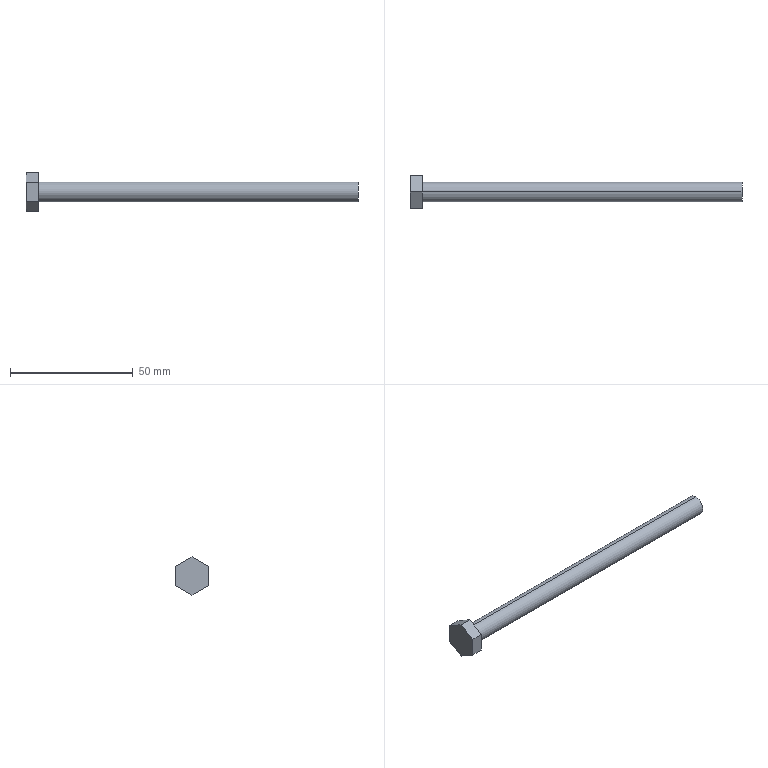Part | SolidWorks | features BaseBody 1 | 1 solid | 11 faces | box 135 x 13.5 x 15.588 mm | volume 7324 mm3 | plane 9 | cylinder 2 | commonest cylinder face diameters 8 x2
STEP:
#1=CARTESIAN_POINT('',(135.,0.,4.));
#2=VERTEX_POINT('',#1);
#3=CARTESIAN_POINT('',(135.,0.,-4.));
#4=VERTEX_POINT('',#3);
#5=CARTESIAN_POINT('',(135.,0.,0.));
#6=DIRECTION('',(-1.,0.,0.));
#7=DIRECTION('',(0.,0.,1.));
#8=AXIS2_PLACEMENT_3D('',#5,#6,#7);
#9=CIRCLE('',#8,4.);
#10=EDGE_CURVE('',#2,#4,#9,.T.);
#11=ORIENTED_EDGE('',*,*,#10,.T.);
#12=CARTESIAN_POINT('',(5.,0.,-4.));
#13=VERTEX_POINT('',#12);
#14=CARTESIAN_POINT('',(135.,0.,-4.));
#15=DIRECTION('',(-1.,0.,0.));
#16=VECTOR('',#15,1000.);
#17=LINE('',#14,#16);
#18=EDGE_CURVE('',#4,#13,#17,.T.);
#19=ORIENTED_EDGE('',*,*,#18,.T.);
#20=CARTESIAN_POINT('',(5.,0.,4.));
#21=VERTEX_POINT('',#20);
#22=CARTESIAN_POINT('',(5.,0.,0.));
#23=DIRECTION('',(1.,0.,0.));
#24=DIRECTION('',(0.,0.,1.));
#25=AXIS2_PLACEMENT_3D('',#22,#23,#24);
#26=CIRCLE('',#25,4.);
#27=EDGE_CURVE('',#13,#21,#26,.T.);
#28=ORIENTED_EDGE('',*,*,#27,.T.);
#29=CARTESIAN_POINT('',(135.,0.,4.));
#30=DIRECTION('',(-1.,0.,0.));
#31=VECTOR('',#30,1000.);
#32=LINE('',#29,#31);
#33=EDGE_CURVE('',#2,#21,#32,.T.);
#34=ORIENTED_EDGE('',*,*,#33,.F.);
#35=EDGE_LOOP('',(#11,#19,#28,#34));
#36=FACE_OUTER_BOUND('',#35,.T.);
#37=CARTESIAN_POINT('',(135.,0.,0.));
#38=DIRECTION('',(-1.,0.,0.));
#39=DIRECTION('',(0.,0.,1.));
#40=AXIS2_PLACEMENT_3D('',#37,#38,#39);
#41=CYLINDRICAL_SURFACE('',#40,4.);
#42=ADVANCED_FACE('',(#36),#41,.T.);
#43=ORIENTED_EDGE('',*,*,#18,.F.);
#44=CARTESIAN_POINT('',(135.,0.,0.));
#45=DIRECTION('',(-1.,0.,0.));
#46=DIRECTION('',(0.,0.,1.));
#47=AXIS2_PLACEMENT_3D('',#44,#45,#46);
#48=CIRCLE('',#47,4.);
#49=EDGE_CURVE('',#4,#2,#48,.T.);
#50=ORIENTED_EDGE('',*,*,#49,.T.);
#51=ORIENTED_EDGE('',*,*,#33,.T.);
#52=CARTESIAN_POINT('',(5.,0.,0.));
#53=DIRECTION('',(1.,0.,0.));
#54=DIRECTION('',(0.,0.,1.));
#55=AXIS2_PLACEMENT_3D('',#52,#53,#54);
#56=CIRCLE('',#55,4.);
#57=EDGE_CURVE('',#21,#13,#56,.T.);
#58=ORIENTED_EDGE('',*,*,#57,.T.);
#59=EDGE_LOOP('',(#43,#50,#51,#58));
#60=FACE_OUTER_BOUND('',#59,.T.);
#61=CARTESIAN_POINT('',(135.,0.,0.));
#62=DIRECTION('',(-1.,0.,0.));
#63=DIRECTION('',(0.,0.,1.));
#64=AXIS2_PLACEMENT_3D('',#61,#62,#63);
#65=CYLINDRICAL_SURFACE('',#64,4.);
#66=ADVANCED_FACE('',(#60),#65,.T.);
#67=CARTESIAN_POINT('',(5.,0.,7.794));
#68=VERTEX_POINT('',#67);
#69=CARTESIAN_POINT('',(5.,-6.75,3.897));
#70=VERTEX_POINT('',#69);
#71=CARTESIAN_POINT('',(5.,0.,7.794));
#72=DIRECTION('',(0.,-0.866,-0.5));
#73=VECTOR('',#72,1000.);
#74=LINE('',#71,#73);
#75=EDGE_CURVE('',#68,#70,#74,.T.);
#76=ORIENTED_EDGE('',*,*,#75,.T.);
#77=CARTESIAN_POINT('',(5.,-6.75,-3.897));
#78=VERTEX_POINT('',#77);
#79=CARTESIAN_POINT('',(5.,-6.75,0.));
#80=DIRECTION('',(0.,0.,-1.));
#81=VECTOR('',#80,1000.);
#82=LINE('',#79,#81);
#83=EDGE_CURVE('',#70,#78,#82,.T.);
#84=ORIENTED_EDGE('',*,*,#83,.T.);
#85=CARTESIAN_POINT('',(5.,0.,-7.794));
#86=VERTEX_POINT('',#85);
#87=CARTESIAN_POINT('',(5.,-6.75,-3.897));
#88=DIRECTION('',(0.,0.866,-0.5));
#89=VECTOR('',#88,1000.);
#90=LINE('',#87,#89);
#91=EDGE_CURVE('',#78,#86,#90,.T.);
#92=ORIENTED_EDGE('',*,*,#91,.T.);
#93=CARTESIAN_POINT('',(5.,6.75,-3.897));
#94=VERTEX_POINT('',#93);
#95=CARTESIAN_POINT('',(5.,0.,-7.794));
#96=DIRECTION('',(0.,0.866,0.5));
#97=VECTOR('',#96,1000.);
#98=LINE('',#95,#97);
#99=EDGE_CURVE('',#86,#94,#98,.T.);
#100=ORIENTED_EDGE('',*,*,#99,.T.);
#101=CARTESIAN_POINT('',(5.,6.75,3.897));
#102=VERTEX_POINT('',#101);
#103=CARTESIAN_POINT('',(5.,6.75,0.));
#104=DIRECTION('',(0.,0.,1.));
#105=VECTOR('',#104,1000.);
#106=LINE('',#103,#105);
#107=EDGE_CURVE('',#94,#102,#106,.T.);
#108=ORIENTED_EDGE('',*,*,#107,.T.);
#109=CARTESIAN_POINT('',(5.,6.75,3.897));
#110=DIRECTION('',(0.,-0.866,0.5));
#111=VECTOR('',#110,1000.);
#112=LINE('',#109,#111);
#113=EDGE_CURVE('',#102,#68,#112,.T.);
#114=ORIENTED_EDGE('',*,*,#113,.T.);
#115=EDGE_LOOP('',(#76,#84,#92,#100,#108,#114));
#116=FACE_OUTER_BOUND('',#115,.T.);
#117=ORIENTED_EDGE('',*,*,#57,.F.);
#118=ORIENTED_EDGE('',*,*,#27,.F.);
#119=EDGE_LOOP('',(#117,#118));
#120=FACE_BOUND('',#119,.T.);
#121=CARTESIAN_POINT('',(5.,0.,0.));
#122=DIRECTION('',(1.,0.,0.));
#123=DIRECTION('',(0.,0.,-1.));
#124=AXIS2_PLACEMENT_3D('',#121,#122,#123);
#125=PLANE('',#124);
#126=ADVANCED_FACE('',(#116,#120),#125,.T.);
#127=ORIENTED_EDGE('',*,*,#10,.F.);
#128=ORIENTED_EDGE('',*,*,#49,.F.);
#129=EDGE_LOOP('',(#127,#128));
#130=FACE_OUTER_BOUND('',#129,.T.);
#131=CARTESIAN_POINT('',(135.,0.,0.));
#132=DIRECTION('',(1.,0.,0.));
#133=DIRECTION('',(0.,0.,-1.));
#134=AXIS2_PLACEMENT_3D('',#131,#132,#133);
#135=PLANE('',#134);
#136=ADVANCED_FACE('',(#130),#135,.T.);
#137=CARTESIAN_POINT('',(0.,-6.75,-3.897));
#138=VERTEX_POINT('',#137);
#139=CARTESIAN_POINT('',(5.,-6.75,-3.897));
#140=DIRECTION('',(-1.,0.,0.));
#141=VECTOR('',#140,1000.);
#142=LINE('',#139,#141);
#143=EDGE_CURVE('',#78,#138,#142,.T.);
#144=ORIENTED_EDGE('',*,*,#143,.F.);
#145=ORIENTED_EDGE('',*,*,#83,.F.);
#146=CARTESIAN_POINT('',(0.,-6.75,3.897));
#147=VERTEX_POINT('',#146);
#148=CARTESIAN_POINT('',(5.,-6.75,3.897));
#149=DIRECTION('',(1.,0.,0.));
#150=VECTOR('',#149,1000.);
#151=LINE('',#148,#150);
#152=EDGE_CURVE('',#147,#70,#151,.T.);
#153=ORIENTED_EDGE('',*,*,#152,.F.);
#154=CARTESIAN_POINT('',(0.,-6.75,3.897));
#155=DIRECTION('',(0.,0.,1.));
#156=VECTOR('',#155,1000.);
#157=LINE('',#154,#156);
#158=EDGE_CURVE('',#138,#147,#157,.T.);
#159=ORIENTED_EDGE('',*,*,#158,.F.);
#160=EDGE_LOOP('',(#144,#145,#153,#159));
#161=FACE_OUTER_BOUND('',#160,.T.);
#162=CARTESIAN_POINT('',(5.,-6.75,3.897));
#163=DIRECTION('',(0.,1.,0.));
#164=DIRECTION('',(0.,0.,1.));
#165=AXIS2_PLACEMENT_3D('',#162,#163,#164);
#166=PLANE('',#165);
#167=ADVANCED_FACE('',(#161),#166,.F.);
#168=ORIENTED_EDGE('',*,*,#152,.T.);
#169=ORIENTED_EDGE('',*,*,#75,.F.);
#170=CARTESIAN_POINT('',(0.,0.,7.794));
#171=VERTEX_POINT('',#170);
#172=CARTESIAN_POINT('',(5.,0.,7.794));
#173=DIRECTION('',(1.,0.,0.));
#174=VECTOR('',#173,1000.);
#175=LINE('',#172,#174);
#176=EDGE_CURVE('',#171,#68,#175,.T.);
#177=ORIENTED_EDGE('',*,*,#176,.F.);
#178=CARTESIAN_POINT('',(0.,0.,7.794));
#179=DIRECTION('',(0.,0.866,0.5));
#180=VECTOR('',#179,1000.);
#181=LINE('',#178,#180);
#182=EDGE_CURVE('',#147,#171,#181,.T.);
#183=ORIENTED_EDGE('',*,*,#182,.F.);
#184=EDGE_LOOP('',(#168,#169,#177,#183));
#185=FACE_OUTER_BOUND('',#184,.T.);
#186=CARTESIAN_POINT('',(5.,0.,7.794));
#187=DIRECTION('',(0.,0.5,-0.866));
#188=DIRECTION('',(0.,0.866,0.5));
#189=AXIS2_PLACEMENT_3D('',#186,#187,#188);
#190=PLANE('',#189);
#191=ADVANCED_FACE('',(#185),#190,.F.);
#192=ORIENTED_EDGE('',*,*,#176,.T.);
#193=ORIENTED_EDGE('',*,*,#113,.F.);
#194=CARTESIAN_POINT('',(0.,6.75,3.897));
#195=VERTEX_POINT('',#194);
#196=CARTESIAN_POINT('',(5.,6.75,3.897));
#197=DIRECTION('',(1.,0.,0.));
#198=VECTOR('',#197,1000.);
#199=LINE('',#196,#198);
#200=EDGE_CURVE('',#195,#102,#199,.T.);
#201=ORIENTED_EDGE('',*,*,#200,.F.);
#202=CARTESIAN_POINT('',(0.,6.75,3.897));
#203=DIRECTION('',(0.,0.866,-0.5));
#204=VECTOR('',#203,1000.);
#205=LINE('',#202,#204);
#206=EDGE_CURVE('',#171,#195,#205,.T.);
#207=ORIENTED_EDGE('',*,*,#206,.F.);
#208=EDGE_LOOP('',(#192,#193,#201,#207));
#209=FACE_OUTER_BOUND('',#208,.T.);
#210=CARTESIAN_POINT('',(5.,6.75,3.897));
#211=DIRECTION('',(0.,-0.5,-0.866));
#212=DIRECTION('',(0.,0.866,-0.5));
#213=AXIS2_PLACEMENT_3D('',#210,#211,#212);
#214=PLANE('',#213);
#215=ADVANCED_FACE('',(#209),#214,.F.);
#216=ORIENTED_EDGE('',*,*,#200,.T.);
#217=ORIENTED_EDGE('',*,*,#107,.F.);
#218=CARTESIAN_POINT('',(0.,6.75,-3.897));
#219=VERTEX_POINT('',#218);
#220=CARTESIAN_POINT('',(5.,6.75,-3.897));
#221=DIRECTION('',(1.,0.,0.));
#222=VECTOR('',#221,1000.);
#223=LINE('',#220,#222);
#224=EDGE_CURVE('',#219,#94,#223,.T.);
#225=ORIENTED_EDGE('',*,*,#224,.F.);
#226=CARTESIAN_POINT('',(0.,6.75,-3.897));
#227=DIRECTION('',(0.,0.,-1.));
#228=VECTOR('',#227,1000.);
#229=LINE('',#226,#228);
#230=EDGE_CURVE('',#195,#219,#229,.T.);
#231=ORIENTED_EDGE('',*,*,#230,.F.);
#232=EDGE_LOOP('',(#216,#217,#225,#231));
#233=FACE_OUTER_BOUND('',#232,.T.);
#234=CARTESIAN_POINT('',(5.,6.75,-3.897));
#235=DIRECTION('',(0.,-1.,0.));
#236=DIRECTION('',(0.,0.,-1.));
#237=AXIS2_PLACEMENT_3D('',#234,#235,#236);
#238=PLANE('',#237);
#239=ADVANCED_FACE('',(#233),#238,.F.);
#240=ORIENTED_EDGE('',*,*,#224,.T.);
#241=ORIENTED_EDGE('',*,*,#99,.F.);
#242=CARTESIAN_POINT('',(0.,0.,-7.794));
#243=VERTEX_POINT('',#242);
#244=CARTESIAN_POINT('',(5.,0.,-7.794));
#245=DIRECTION('',(1.,0.,0.));
#246=VECTOR('',#245,1000.);
#247=LINE('',#244,#246);
#248=EDGE_CURVE('',#243,#86,#247,.T.);
#249=ORIENTED_EDGE('',*,*,#248,.F.);
#250=CARTESIAN_POINT('',(0.,0.,-7.794));
#251=DIRECTION('',(0.,-0.866,-0.5));
#252=VECTOR('',#251,1000.);
#253=LINE('',#250,#252);
#254=EDGE_CURVE('',#219,#243,#253,.T.);
#255=ORIENTED_EDGE('',*,*,#254,.F.);
#256=EDGE_LOOP('',(#240,#241,#249,#255));
#257=FACE_OUTER_BOUND('',#256,.T.);
#258=CARTESIAN_POINT('',(5.,0.,-7.794));
#259=DIRECTION('',(0.,-0.5,0.866));
#260=DIRECTION('',(0.,-0.866,-0.5));
#261=AXIS2_PLACEMENT_3D('',#258,#259,#260);
#262=PLANE('',#261);
#263=ADVANCED_FACE('',(#257),#262,.F.);
#264=ORIENTED_EDGE('',*,*,#248,.T.);
#265=ORIENTED_EDGE('',*,*,#91,.F.);
#266=ORIENTED_EDGE('',*,*,#143,.T.);
#267=CARTESIAN_POINT('',(0.,-6.75,-3.897));
#268=DIRECTION('',(0.,-0.866,0.5));
#269=VECTOR('',#268,1000.);
#270=LINE('',#267,#269);
#271=EDGE_CURVE('',#243,#138,#270,.T.);
#272=ORIENTED_EDGE('',*,*,#271,.F.);
#273=EDGE_LOOP('',(#264,#265,#266,#272));
#274=FACE_OUTER_BOUND('',#273,.T.);
#275=CARTESIAN_POINT('',(5.,-6.75,-3.897));
#276=DIRECTION('',(0.,0.5,0.866));
#277=DIRECTION('',(0.,-0.866,0.5));
#278=AXIS2_PLACEMENT_3D('',#275,#276,#277);
#279=PLANE('',#278);
#280=ADVANCED_FACE('',(#274),#279,.F.);
#281=ORIENTED_EDGE('',*,*,#158,.T.);
#282=ORIENTED_EDGE('',*,*,#182,.T.);
#283=ORIENTED_EDGE('',*,*,#206,.T.);
#284=ORIENTED_EDGE('',*,*,#230,.T.);
#285=ORIENTED_EDGE('',*,*,#254,.T.);
#286=ORIENTED_EDGE('',*,*,#271,.T.);
#287=EDGE_LOOP('',(#281,#282,#283,#284,#285,#286));
#288=FACE_OUTER_BOUND('',#287,.T.);
#289=CARTESIAN_POINT('',(0.,0.,0.));
#290=DIRECTION('',(1.,0.,0.));
#291=DIRECTION('',(0.,0.,-1.));
#292=AXIS2_PLACEMENT_3D('',#289,#290,#291);
#293=PLANE('',#292);
#294=ADVANCED_FACE('',(#288),#293,.F.);
#295=CLOSED_SHELL('',(#42,#66,#126,#136,#167,#191,#215,#239,#263,#280,#294));
#296=MANIFOLD_SOLID_BREP('',#295);
#297=CARTESIAN_POINT('',(0.,0.,0.));
#298=DIRECTION('',(0.,0.,1.));
#299=DIRECTION('',(1.,0.,0.));
#300=AXIS2_PLACEMENT_3D('',#297,#298,#299);
#301=(LENGTH_UNIT()NAMED_UNIT(*)SI_UNIT(.MILLI.,.METRE.));
#302=UNCERTAINTY_MEASURE_WITH_UNIT(LENGTH_MEASURE(0.00001),#301,'','');
#303=(NAMED_UNIT(*)PLANE_ANGLE_UNIT()SI_UNIT($,.RADIAN.));
#304=(NAMED_UNIT(*)SI_UNIT($,.STERADIAN.)SOLID_ANGLE_UNIT());
#305=(GEOMETRIC_REPRESENTATION_CONTEXT(3)GLOBAL_UNCERTAINTY_ASSIGNED_CONTEXT((#302))GLOBAL_UNIT_ASSIGNED_CONTEXT((#301,#303,#304))REPRESENTATION_CONTEXT('',''));
#306=ADVANCED_BREP_SHAPE_REPRESENTATION('',(#296,#300),#305);